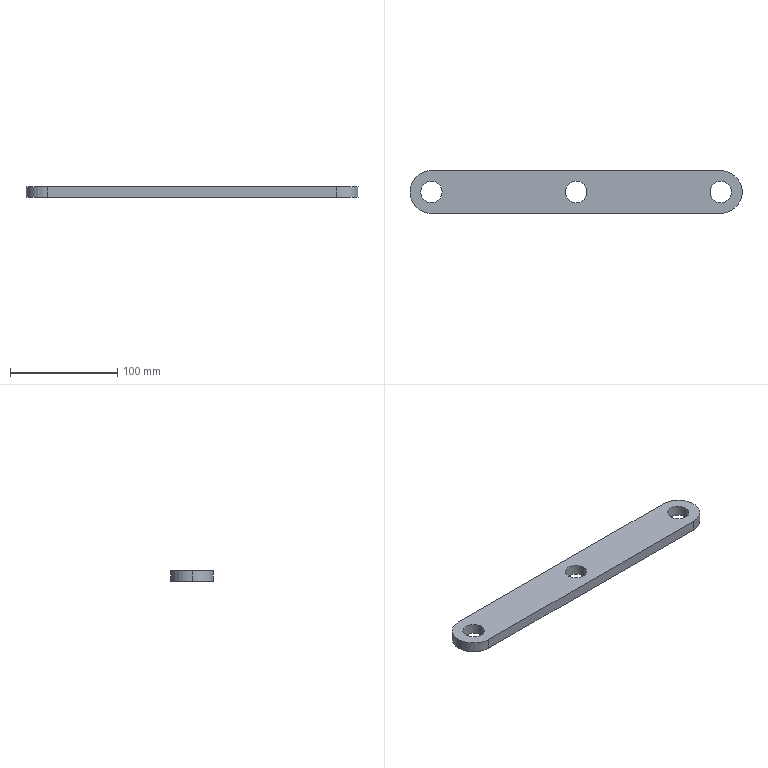Part | SolidWorks | features ICE 2, Extrusion 1 | 1 solid | 13 faces | box 310 x 40 x 10 mm | volume 111142 mm3 | cylinder 9 | plane 4 | commonest cylinder face diameters 20 x6 40 x3
STEP:
#1=CARTESIAN_POINT('',(-10.,0.,0.));
#2=VERTEX_POINT('',#1);
#3=CARTESIAN_POINT('',(10.,0.,0.));
#4=VERTEX_POINT('',#3);
#5=CARTESIAN_POINT('',(0.,0.,0.));
#6=DIRECTION('',(0.,0.,1.));
#7=DIRECTION('',(1.,0.,0.));
#8=AXIS2_PLACEMENT_3D('',#5,#6,#7);
#9=CIRCLE('',#8,10.);
#10=EDGE_CURVE('',#2,#4,#9,.T.);
#11=ORIENTED_EDGE('',*,*,#10,.F.);
#12=CARTESIAN_POINT('',(-10.,0.,10.));
#13=VERTEX_POINT('',#12);
#14=CARTESIAN_POINT('',(-10.,0.,0.));
#15=DIRECTION('',(0.,0.,1.));
#16=VECTOR('',#15,1000.);
#17=LINE('',#14,#16);
#18=EDGE_CURVE('',#2,#13,#17,.T.);
#19=ORIENTED_EDGE('',*,*,#18,.T.);
#20=CARTESIAN_POINT('',(10.,0.,10.));
#21=VERTEX_POINT('',#20);
#22=CARTESIAN_POINT('',(0.,0.,10.));
#23=DIRECTION('',(0.,0.,1.));
#24=DIRECTION('',(1.,0.,0.));
#25=AXIS2_PLACEMENT_3D('',#22,#23,#24);
#26=CIRCLE('',#25,10.);
#27=EDGE_CURVE('',#13,#21,#26,.T.);
#28=ORIENTED_EDGE('',*,*,#27,.T.);
#29=CARTESIAN_POINT('',(10.,0.,0.));
#30=DIRECTION('',(0.,0.,1.));
#31=VECTOR('',#30,1000.);
#32=LINE('',#29,#31);
#33=EDGE_CURVE('',#4,#21,#32,.T.);
#34=ORIENTED_EDGE('',*,*,#33,.F.);
#35=EDGE_LOOP('',(#11,#19,#28,#34));
#36=FACE_OUTER_BOUND('',#35,.T.);
#37=CARTESIAN_POINT('',(0.,0.,0.));
#38=DIRECTION('',(0.,0.,1.));
#39=DIRECTION('',(1.,0.,0.));
#40=AXIS2_PLACEMENT_3D('',#37,#38,#39);
#41=CYLINDRICAL_SURFACE('',#40,10.);
#42=ADVANCED_FACE('',(#36),#41,.F.);
#43=CARTESIAN_POINT('',(-145.,0.,0.));
#44=VERTEX_POINT('',#43);
#45=CARTESIAN_POINT('',(-125.,0.,0.));
#46=VERTEX_POINT('',#45);
#47=CARTESIAN_POINT('',(-135.,0.,0.));
#48=DIRECTION('',(0.,0.,1.));
#49=DIRECTION('',(1.,0.,0.));
#50=AXIS2_PLACEMENT_3D('',#47,#48,#49);
#51=CIRCLE('',#50,10.);
#52=EDGE_CURVE('',#44,#46,#51,.T.);
#53=ORIENTED_EDGE('',*,*,#52,.F.);
#54=CARTESIAN_POINT('',(-145.,0.,10.));
#55=VERTEX_POINT('',#54);
#56=CARTESIAN_POINT('',(-145.,0.,0.));
#57=DIRECTION('',(0.,0.,1.));
#58=VECTOR('',#57,1000.);
#59=LINE('',#56,#58);
#60=EDGE_CURVE('',#44,#55,#59,.T.);
#61=ORIENTED_EDGE('',*,*,#60,.T.);
#62=CARTESIAN_POINT('',(-125.,0.,10.));
#63=VERTEX_POINT('',#62);
#64=CARTESIAN_POINT('',(-135.,0.,10.));
#65=DIRECTION('',(0.,0.,1.));
#66=DIRECTION('',(1.,0.,0.));
#67=AXIS2_PLACEMENT_3D('',#64,#65,#66);
#68=CIRCLE('',#67,10.);
#69=EDGE_CURVE('',#55,#63,#68,.T.);
#70=ORIENTED_EDGE('',*,*,#69,.T.);
#71=CARTESIAN_POINT('',(-125.,0.,0.));
#72=DIRECTION('',(0.,0.,1.));
#73=VECTOR('',#72,1000.);
#74=LINE('',#71,#73);
#75=EDGE_CURVE('',#46,#63,#74,.T.);
#76=ORIENTED_EDGE('',*,*,#75,.F.);
#77=EDGE_LOOP('',(#53,#61,#70,#76));
#78=FACE_OUTER_BOUND('',#77,.T.);
#79=CARTESIAN_POINT('',(-135.,0.,0.));
#80=DIRECTION('',(0.,0.,1.));
#81=DIRECTION('',(1.,0.,0.));
#82=AXIS2_PLACEMENT_3D('',#79,#80,#81);
#83=CYLINDRICAL_SURFACE('',#82,10.);
#84=ADVANCED_FACE('',(#78),#83,.F.);
#85=CARTESIAN_POINT('',(125.,0.,0.));
#86=VERTEX_POINT('',#85);
#87=CARTESIAN_POINT('',(145.,0.,0.));
#88=VERTEX_POINT('',#87);
#89=CARTESIAN_POINT('',(135.,0.,0.));
#90=DIRECTION('',(0.,0.,1.));
#91=DIRECTION('',(1.,0.,0.));
#92=AXIS2_PLACEMENT_3D('',#89,#90,#91);
#93=CIRCLE('',#92,10.);
#94=EDGE_CURVE('',#86,#88,#93,.T.);
#95=ORIENTED_EDGE('',*,*,#94,.F.);
#96=CARTESIAN_POINT('',(125.,0.,10.));
#97=VERTEX_POINT('',#96);
#98=CARTESIAN_POINT('',(125.,0.,0.));
#99=DIRECTION('',(0.,0.,1.));
#100=VECTOR('',#99,1000.);
#101=LINE('',#98,#100);
#102=EDGE_CURVE('',#86,#97,#101,.T.);
#103=ORIENTED_EDGE('',*,*,#102,.T.);
#104=CARTESIAN_POINT('',(145.,0.,10.));
#105=VERTEX_POINT('',#104);
#106=CARTESIAN_POINT('',(135.,0.,10.));
#107=DIRECTION('',(0.,0.,1.));
#108=DIRECTION('',(1.,0.,0.));
#109=AXIS2_PLACEMENT_3D('',#106,#107,#108);
#110=CIRCLE('',#109,10.);
#111=EDGE_CURVE('',#97,#105,#110,.T.);
#112=ORIENTED_EDGE('',*,*,#111,.T.);
#113=CARTESIAN_POINT('',(145.,0.,0.));
#114=DIRECTION('',(0.,0.,1.));
#115=VECTOR('',#114,1000.);
#116=LINE('',#113,#115);
#117=EDGE_CURVE('',#88,#105,#116,.T.);
#118=ORIENTED_EDGE('',*,*,#117,.F.);
#119=EDGE_LOOP('',(#95,#103,#112,#118));
#120=FACE_OUTER_BOUND('',#119,.T.);
#121=CARTESIAN_POINT('',(135.,0.,0.));
#122=DIRECTION('',(0.,0.,1.));
#123=DIRECTION('',(1.,0.,0.));
#124=AXIS2_PLACEMENT_3D('',#121,#122,#123);
#125=CYLINDRICAL_SURFACE('',#124,10.);
#126=ADVANCED_FACE('',(#120),#125,.F.);
#127=CARTESIAN_POINT('',(-155.,0.,10.));
#128=VERTEX_POINT('',#127);
#129=CARTESIAN_POINT('',(-135.,-20.,10.));
#130=VERTEX_POINT('',#129);
#131=CARTESIAN_POINT('',(-135.,0.,10.));
#132=DIRECTION('',(0.,0.,1.));
#133=DIRECTION('',(1.,0.,0.));
#134=AXIS2_PLACEMENT_3D('',#131,#132,#133);
#135=CIRCLE('',#134,20.);
#136=EDGE_CURVE('',#128,#130,#135,.T.);
#137=ORIENTED_EDGE('',*,*,#136,.F.);
#138=CARTESIAN_POINT('',(-155.,0.,0.));
#139=VERTEX_POINT('',#138);
#140=CARTESIAN_POINT('',(-155.,0.,10.));
#141=DIRECTION('',(0.,0.,-1.));
#142=VECTOR('',#141,1000.);
#143=LINE('',#140,#142);
#144=EDGE_CURVE('',#128,#139,#143,.T.);
#145=ORIENTED_EDGE('',*,*,#144,.T.);
#146=CARTESIAN_POINT('',(-135.,-20.,0.));
#147=VERTEX_POINT('',#146);
#148=CARTESIAN_POINT('',(-135.,0.,0.));
#149=DIRECTION('',(0.,0.,1.));
#150=DIRECTION('',(1.,0.,0.));
#151=AXIS2_PLACEMENT_3D('',#148,#149,#150);
#152=CIRCLE('',#151,20.);
#153=EDGE_CURVE('',#139,#147,#152,.T.);
#154=ORIENTED_EDGE('',*,*,#153,.T.);
#155=CARTESIAN_POINT('',(-135.,-20.,10.));
#156=DIRECTION('',(0.,0.,-1.));
#157=VECTOR('',#156,1000.);
#158=LINE('',#155,#157);
#159=EDGE_CURVE('',#130,#147,#158,.T.);
#160=ORIENTED_EDGE('',*,*,#159,.F.);
#161=EDGE_LOOP('',(#137,#145,#154,#160));
#162=FACE_OUTER_BOUND('',#161,.T.);
#163=CARTESIAN_POINT('',(-135.,0.,10.));
#164=DIRECTION('',(0.,0.,-1.));
#165=DIRECTION('',(-1.,0.,0.));
#166=AXIS2_PLACEMENT_3D('',#163,#164,#165);
#167=CYLINDRICAL_SURFACE('',#166,20.);
#168=ADVANCED_FACE('',(#162),#167,.T.);
#169=ORIENTED_EDGE('',*,*,#144,.F.);
#170=CARTESIAN_POINT('',(-135.,20.,10.));
#171=VERTEX_POINT('',#170);
#172=CARTESIAN_POINT('',(-135.,0.,10.));
#173=DIRECTION('',(0.,0.,1.));
#174=DIRECTION('',(1.,0.,0.));
#175=AXIS2_PLACEMENT_3D('',#172,#173,#174);
#176=CIRCLE('',#175,20.);
#177=EDGE_CURVE('',#171,#128,#176,.T.);
#178=ORIENTED_EDGE('',*,*,#177,.F.);
#179=CARTESIAN_POINT('',(-135.,20.,0.));
#180=VERTEX_POINT('',#179);
#181=CARTESIAN_POINT('',(-135.,20.,10.));
#182=DIRECTION('',(0.,0.,-1.));
#183=VECTOR('',#182,1000.);
#184=LINE('',#181,#183);
#185=EDGE_CURVE('',#171,#180,#184,.T.);
#186=ORIENTED_EDGE('',*,*,#185,.T.);
#187=CARTESIAN_POINT('',(-135.,0.,0.));
#188=DIRECTION('',(0.,0.,1.));
#189=DIRECTION('',(1.,0.,0.));
#190=AXIS2_PLACEMENT_3D('',#187,#188,#189);
#191=CIRCLE('',#190,20.);
#192=EDGE_CURVE('',#180,#139,#191,.T.);
#193=ORIENTED_EDGE('',*,*,#192,.T.);
#194=EDGE_LOOP('',(#169,#178,#186,#193));
#195=FACE_OUTER_BOUND('',#194,.T.);
#196=CARTESIAN_POINT('',(-135.,0.,10.));
#197=DIRECTION('',(0.,0.,-1.));
#198=DIRECTION('',(-1.,0.,0.));
#199=AXIS2_PLACEMENT_3D('',#196,#197,#198);
#200=CYLINDRICAL_SURFACE('',#199,20.);
#201=ADVANCED_FACE('',(#195),#200,.T.);
#202=CARTESIAN_POINT('',(135.,-20.,0.));
#203=VERTEX_POINT('',#202);
#204=CARTESIAN_POINT('',(-135.,-20.,0.));
#205=DIRECTION('',(1.,0.,0.));
#206=VECTOR('',#205,1000.);
#207=LINE('',#204,#206);
#208=EDGE_CURVE('',#147,#203,#207,.T.);
#209=ORIENTED_EDGE('',*,*,#208,.T.);
#210=CARTESIAN_POINT('',(135.,-20.,10.));
#211=VERTEX_POINT('',#210);
#212=CARTESIAN_POINT('',(135.,-20.,10.));
#213=DIRECTION('',(0.,0.,-1.));
#214=VECTOR('',#213,1000.);
#215=LINE('',#212,#214);
#216=EDGE_CURVE('',#211,#203,#215,.T.);
#217=ORIENTED_EDGE('',*,*,#216,.F.);
#218=CARTESIAN_POINT('',(-135.,-20.,10.));
#219=DIRECTION('',(1.,0.,0.));
#220=VECTOR('',#219,1000.);
#221=LINE('',#218,#220);
#222=EDGE_CURVE('',#130,#211,#221,.T.);
#223=ORIENTED_EDGE('',*,*,#222,.F.);
#224=ORIENTED_EDGE('',*,*,#159,.T.);
#225=EDGE_LOOP('',(#209,#217,#223,#224));
#226=FACE_OUTER_BOUND('',#225,.T.);
#227=CARTESIAN_POINT('',(-135.,-20.,10.));
#228=DIRECTION('',(0.,1.,0.));
#229=DIRECTION('',(0.,0.,1.));
#230=AXIS2_PLACEMENT_3D('',#227,#228,#229);
#231=PLANE('',#230);
#232=ADVANCED_FACE('',(#226),#231,.F.);
#233=CARTESIAN_POINT('',(135.,20.,0.));
#234=VERTEX_POINT('',#233);
#235=CARTESIAN_POINT('',(135.,0.,0.));
#236=DIRECTION('',(0.,0.,1.));
#237=DIRECTION('',(1.,0.,0.));
#238=AXIS2_PLACEMENT_3D('',#235,#236,#237);
#239=CIRCLE('',#238,20.);
#240=EDGE_CURVE('',#203,#234,#239,.T.);
#241=ORIENTED_EDGE('',*,*,#240,.T.);
#242=CARTESIAN_POINT('',(135.,20.,10.));
#243=VERTEX_POINT('',#242);
#244=CARTESIAN_POINT('',(135.,20.,10.));
#245=DIRECTION('',(0.,0.,-1.));
#246=VECTOR('',#245,1000.);
#247=LINE('',#244,#246);
#248=EDGE_CURVE('',#243,#234,#247,.T.);
#249=ORIENTED_EDGE('',*,*,#248,.F.);
#250=CARTESIAN_POINT('',(135.,0.,10.));
#251=DIRECTION('',(0.,0.,1.));
#252=DIRECTION('',(1.,0.,0.));
#253=AXIS2_PLACEMENT_3D('',#250,#251,#252);
#254=CIRCLE('',#253,20.);
#255=EDGE_CURVE('',#211,#243,#254,.T.);
#256=ORIENTED_EDGE('',*,*,#255,.F.);
#257=ORIENTED_EDGE('',*,*,#216,.T.);
#258=EDGE_LOOP('',(#241,#249,#256,#257));
#259=FACE_OUTER_BOUND('',#258,.T.);
#260=CARTESIAN_POINT('',(135.,0.,10.));
#261=DIRECTION('',(0.,0.,-1.));
#262=DIRECTION('',(-1.,0.,0.));
#263=AXIS2_PLACEMENT_3D('',#260,#261,#262);
#264=CYLINDRICAL_SURFACE('',#263,20.);
#265=ADVANCED_FACE('',(#259),#264,.T.);
#266=CARTESIAN_POINT('',(-135.,20.,0.));
#267=DIRECTION('',(-1.,0.,0.));
#268=VECTOR('',#267,1000.);
#269=LINE('',#266,#268);
#270=EDGE_CURVE('',#234,#180,#269,.T.);
#271=ORIENTED_EDGE('',*,*,#270,.T.);
#272=ORIENTED_EDGE('',*,*,#185,.F.);
#273=CARTESIAN_POINT('',(-135.,20.,10.));
#274=DIRECTION('',(-1.,0.,0.));
#275=VECTOR('',#274,1000.);
#276=LINE('',#273,#275);
#277=EDGE_CURVE('',#243,#171,#276,.T.);
#278=ORIENTED_EDGE('',*,*,#277,.F.);
#279=ORIENTED_EDGE('',*,*,#248,.T.);
#280=EDGE_LOOP('',(#271,#272,#278,#279));
#281=FACE_OUTER_BOUND('',#280,.T.);
#282=CARTESIAN_POINT('',(-135.,20.,10.));
#283=DIRECTION('',(0.,-1.,0.));
#284=DIRECTION('',(1.,0.,0.));
#285=AXIS2_PLACEMENT_3D('',#282,#283,#284);
#286=PLANE('',#285);
#287=ADVANCED_FACE('',(#281),#286,.F.);
#288=CARTESIAN_POINT('',(0.,0.,10.));
#289=DIRECTION('',(0.,0.,1.));
#290=DIRECTION('',(1.,0.,0.));
#291=AXIS2_PLACEMENT_3D('',#288,#289,#290);
#292=CIRCLE('',#291,10.);
#293=EDGE_CURVE('',#21,#13,#292,.T.);
#294=ORIENTED_EDGE('',*,*,#293,.F.);
#295=ORIENTED_EDGE('',*,*,#27,.F.);
#296=EDGE_LOOP('',(#294,#295));
#297=FACE_BOUND('',#296,.T.);
#298=CARTESIAN_POINT('',(-135.,0.,10.));
#299=DIRECTION('',(0.,0.,1.));
#300=DIRECTION('',(1.,0.,0.));
#301=AXIS2_PLACEMENT_3D('',#298,#299,#300);
#302=CIRCLE('',#301,10.);
#303=EDGE_CURVE('',#63,#55,#302,.T.);
#304=ORIENTED_EDGE('',*,*,#303,.F.);
#305=ORIENTED_EDGE('',*,*,#69,.F.);
#306=EDGE_LOOP('',(#304,#305));
#307=FACE_BOUND('',#306,.T.);
#308=CARTESIAN_POINT('',(135.,0.,10.));
#309=DIRECTION('',(0.,0.,1.));
#310=DIRECTION('',(1.,0.,0.));
#311=AXIS2_PLACEMENT_3D('',#308,#309,#310);
#312=CIRCLE('',#311,10.);
#313=EDGE_CURVE('',#105,#97,#312,.T.);
#314=ORIENTED_EDGE('',*,*,#313,.F.);
#315=ORIENTED_EDGE('',*,*,#111,.F.);
#316=EDGE_LOOP('',(#314,#315));
#317=FACE_BOUND('',#316,.T.);
#318=ORIENTED_EDGE('',*,*,#177,.T.);
#319=ORIENTED_EDGE('',*,*,#136,.T.);
#320=ORIENTED_EDGE('',*,*,#222,.T.);
#321=ORIENTED_EDGE('',*,*,#255,.T.);
#322=ORIENTED_EDGE('',*,*,#277,.T.);
#323=EDGE_LOOP('',(#318,#319,#320,#321,#322));
#324=FACE_OUTER_BOUND('',#323,.T.);
#325=CARTESIAN_POINT('',(-135.,0.,10.));
#326=DIRECTION('',(0.,0.,1.));
#327=DIRECTION('',(1.,0.,0.));
#328=AXIS2_PLACEMENT_3D('',#325,#326,#327);
#329=PLANE('',#328);
#330=ADVANCED_FACE('',(#297,#307,#317,#324),#329,.T.);
#331=CARTESIAN_POINT('',(0.,0.,0.));
#332=DIRECTION('',(0.,0.,1.));
#333=DIRECTION('',(1.,0.,0.));
#334=AXIS2_PLACEMENT_3D('',#331,#332,#333);
#335=CIRCLE('',#334,10.);
#336=EDGE_CURVE('',#4,#2,#335,.T.);
#337=ORIENTED_EDGE('',*,*,#336,.T.);
#338=ORIENTED_EDGE('',*,*,#10,.T.);
#339=EDGE_LOOP('',(#337,#338));
#340=FACE_BOUND('',#339,.T.);
#341=CARTESIAN_POINT('',(-135.,0.,0.));
#342=DIRECTION('',(0.,0.,1.));
#343=DIRECTION('',(1.,0.,0.));
#344=AXIS2_PLACEMENT_3D('',#341,#342,#343);
#345=CIRCLE('',#344,10.);
#346=EDGE_CURVE('',#46,#44,#345,.T.);
#347=ORIENTED_EDGE('',*,*,#346,.T.);
#348=ORIENTED_EDGE('',*,*,#52,.T.);
#349=EDGE_LOOP('',(#347,#348));
#350=FACE_BOUND('',#349,.T.);
#351=CARTESIAN_POINT('',(135.,0.,0.));
#352=DIRECTION('',(0.,0.,1.));
#353=DIRECTION('',(1.,0.,0.));
#354=AXIS2_PLACEMENT_3D('',#351,#352,#353);
#355=CIRCLE('',#354,10.);
#356=EDGE_CURVE('',#88,#86,#355,.T.);
#357=ORIENTED_EDGE('',*,*,#356,.T.);
#358=ORIENTED_EDGE('',*,*,#94,.T.);
#359=EDGE_LOOP('',(#357,#358));
#360=FACE_BOUND('',#359,.T.);
#361=ORIENTED_EDGE('',*,*,#192,.F.);
#362=ORIENTED_EDGE('',*,*,#270,.F.);
#363=ORIENTED_EDGE('',*,*,#240,.F.);
#364=ORIENTED_EDGE('',*,*,#208,.F.);
#365=ORIENTED_EDGE('',*,*,#153,.F.);
#366=EDGE_LOOP('',(#361,#362,#363,#364,#365));
#367=FACE_OUTER_BOUND('',#366,.T.);
#368=CARTESIAN_POINT('',(-135.,0.,0.));
#369=DIRECTION('',(0.,0.,1.));
#370=DIRECTION('',(1.,0.,0.));
#371=AXIS2_PLACEMENT_3D('',#368,#369,#370);
#372=PLANE('',#371);
#373=ADVANCED_FACE('',(#340,#350,#360,#367),#372,.F.);
#374=ORIENTED_EDGE('',*,*,#102,.F.);
#375=ORIENTED_EDGE('',*,*,#356,.F.);
#376=ORIENTED_EDGE('',*,*,#117,.T.);
#377=ORIENTED_EDGE('',*,*,#313,.T.);
#378=EDGE_LOOP('',(#374,#375,#376,#377));
#379=FACE_OUTER_BOUND('',#378,.T.);
#380=CARTESIAN_POINT('',(135.,0.,0.));
#381=DIRECTION('',(0.,0.,1.));
#382=DIRECTION('',(1.,0.,0.));
#383=AXIS2_PLACEMENT_3D('',#380,#381,#382);
#384=CYLINDRICAL_SURFACE('',#383,10.);
#385=ADVANCED_FACE('',(#379),#384,.F.);
#386=ORIENTED_EDGE('',*,*,#60,.F.);
#387=ORIENTED_EDGE('',*,*,#346,.F.);
#388=ORIENTED_EDGE('',*,*,#75,.T.);
#389=ORIENTED_EDGE('',*,*,#303,.T.);
#390=EDGE_LOOP('',(#386,#387,#388,#389));
#391=FACE_OUTER_BOUND('',#390,.T.);
#392=CARTESIAN_POINT('',(-135.,0.,0.));
#393=DIRECTION('',(0.,0.,1.));
#394=DIRECTION('',(1.,0.,0.));
#395=AXIS2_PLACEMENT_3D('',#392,#393,#394);
#396=CYLINDRICAL_SURFACE('',#395,10.);
#397=ADVANCED_FACE('',(#391),#396,.F.);
#398=ORIENTED_EDGE('',*,*,#18,.F.);
#399=ORIENTED_EDGE('',*,*,#336,.F.);
#400=ORIENTED_EDGE('',*,*,#33,.T.);
#401=ORIENTED_EDGE('',*,*,#293,.T.);
#402=EDGE_LOOP('',(#398,#399,#400,#401));
#403=FACE_OUTER_BOUND('',#402,.T.);
#404=CARTESIAN_POINT('',(0.,0.,0.));
#405=DIRECTION('',(0.,0.,1.));
#406=DIRECTION('',(1.,0.,0.));
#407=AXIS2_PLACEMENT_3D('',#404,#405,#406);
#408=CYLINDRICAL_SURFACE('',#407,10.);
#409=ADVANCED_FACE('',(#403),#408,.F.);
#410=CLOSED_SHELL('',(#42,#84,#126,#168,#201,#232,#265,#287,#330,#373,#385,#397,#409));
#411=MANIFOLD_SOLID_BREP('',#410);
#412=CARTESIAN_POINT('',(0.,0.,0.));
#413=DIRECTION('',(0.,0.,1.));
#414=DIRECTION('',(1.,0.,0.));
#415=AXIS2_PLACEMENT_3D('',#412,#413,#414);
#416=(LENGTH_UNIT()NAMED_UNIT(*)SI_UNIT(.MILLI.,.METRE.));
#417=UNCERTAINTY_MEASURE_WITH_UNIT(LENGTH_MEASURE(0.00001),#416,'','');
#418=(NAMED_UNIT(*)PLANE_ANGLE_UNIT()SI_UNIT($,.RADIAN.));
#419=(NAMED_UNIT(*)SI_UNIT($,.STERADIAN.)SOLID_ANGLE_UNIT());
#420=(GEOMETRIC_REPRESENTATION_CONTEXT(3)GLOBAL_UNCERTAINTY_ASSIGNED_CONTEXT((#417))GLOBAL_UNIT_ASSIGNED_CONTEXT((#416,#418,#419))REPRESENTATION_CONTEXT('',''));
#421=ADVANCED_BREP_SHAPE_REPRESENTATION('',(#411,#415),#420);